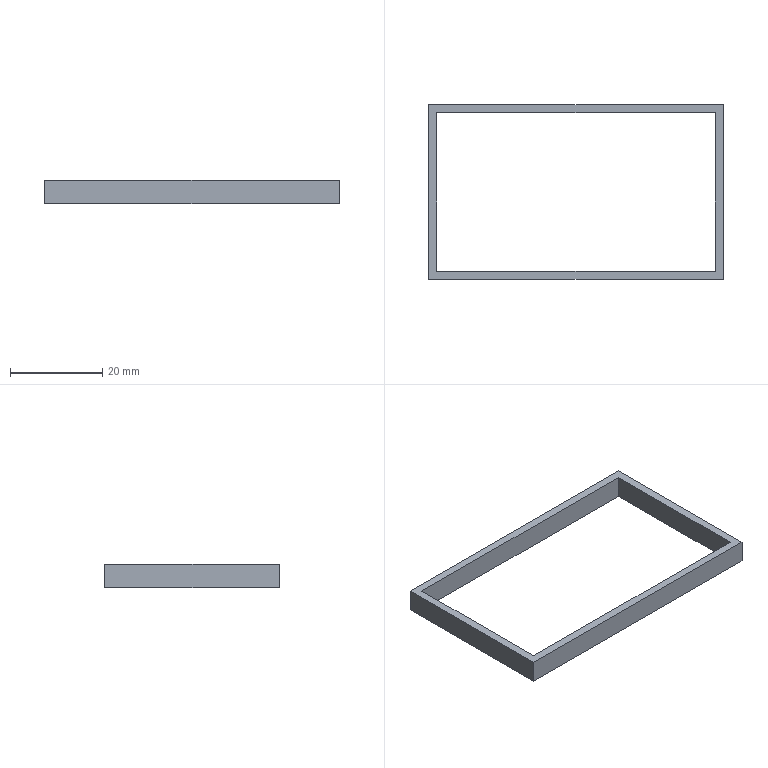Part | SolidWorks | features Extrusion 1 | 1 solid | 10 faces | box 64 x 38 x 5 mm | volume 1771 mm3 | plane 10
STEP:
#1=CARTESIAN_POINT('',(-32.,19.,2.5));
#2=VERTEX_POINT('',#1);
#3=CARTESIAN_POINT('',(-32.,-19.,2.5));
#4=VERTEX_POINT('',#3);
#5=CARTESIAN_POINT('',(-32.,19.,2.5));
#6=DIRECTION('',(0.,-1.,0.));
#7=VECTOR('',#6,1000.);
#8=LINE('',#5,#7);
#9=EDGE_CURVE('',#2,#4,#8,.T.);
#10=ORIENTED_EDGE('',*,*,#9,.F.);
#11=CARTESIAN_POINT('',(-32.,19.,-2.5));
#12=VERTEX_POINT('',#11);
#13=CARTESIAN_POINT('',(-32.,19.,-2.5));
#14=DIRECTION('',(0.,0.,1.));
#15=VECTOR('',#14,1000.);
#16=LINE('',#13,#15);
#17=EDGE_CURVE('',#12,#2,#16,.T.);
#18=ORIENTED_EDGE('',*,*,#17,.F.);
#19=CARTESIAN_POINT('',(-32.,-19.,-2.5));
#20=VERTEX_POINT('',#19);
#21=CARTESIAN_POINT('',(-32.,19.,-2.5));
#22=DIRECTION('',(0.,-1.,0.));
#23=VECTOR('',#22,1000.);
#24=LINE('',#21,#23);
#25=EDGE_CURVE('',#12,#20,#24,.T.);
#26=ORIENTED_EDGE('',*,*,#25,.T.);
#27=CARTESIAN_POINT('',(-32.,-19.,-2.5));
#28=DIRECTION('',(0.,0.,1.));
#29=VECTOR('',#28,1000.);
#30=LINE('',#27,#29);
#31=EDGE_CURVE('',#20,#4,#30,.T.);
#32=ORIENTED_EDGE('',*,*,#31,.T.);
#33=EDGE_LOOP('',(#10,#18,#26,#32));
#34=FACE_OUTER_BOUND('',#33,.T.);
#35=CARTESIAN_POINT('',(-32.,19.,-2.5));
#36=DIRECTION('',(-1.,0.,0.));
#37=DIRECTION('',(0.,0.,1.));
#38=AXIS2_PLACEMENT_3D('',#35,#36,#37);
#39=PLANE('',#38);
#40=ADVANCED_FACE('',(#34),#39,.T.);
#41=CARTESIAN_POINT('',(32.,19.,2.5));
#42=VERTEX_POINT('',#41);
#43=CARTESIAN_POINT('',(32.,19.,2.5));
#44=DIRECTION('',(-1.,0.,0.));
#45=VECTOR('',#44,1000.);
#46=LINE('',#43,#45);
#47=EDGE_CURVE('',#42,#2,#46,.T.);
#48=ORIENTED_EDGE('',*,*,#47,.F.);
#49=CARTESIAN_POINT('',(32.,19.,-2.5));
#50=VERTEX_POINT('',#49);
#51=CARTESIAN_POINT('',(32.,19.,-2.5));
#52=DIRECTION('',(0.,0.,1.));
#53=VECTOR('',#52,1000.);
#54=LINE('',#51,#53);
#55=EDGE_CURVE('',#50,#42,#54,.T.);
#56=ORIENTED_EDGE('',*,*,#55,.F.);
#57=CARTESIAN_POINT('',(32.,19.,-2.5));
#58=DIRECTION('',(-1.,0.,0.));
#59=VECTOR('',#58,1000.);
#60=LINE('',#57,#59);
#61=EDGE_CURVE('',#50,#12,#60,.T.);
#62=ORIENTED_EDGE('',*,*,#61,.T.);
#63=ORIENTED_EDGE('',*,*,#17,.T.);
#64=EDGE_LOOP('',(#48,#56,#62,#63));
#65=FACE_OUTER_BOUND('',#64,.T.);
#66=CARTESIAN_POINT('',(32.,19.,-2.5));
#67=DIRECTION('',(0.,1.,0.));
#68=DIRECTION('',(0.,0.,1.));
#69=AXIS2_PLACEMENT_3D('',#66,#67,#68);
#70=PLANE('',#69);
#71=ADVANCED_FACE('',(#65),#70,.T.);
#72=CARTESIAN_POINT('',(32.,-19.,2.5));
#73=VERTEX_POINT('',#72);
#74=CARTESIAN_POINT('',(32.,-19.,2.5));
#75=DIRECTION('',(0.,1.,0.));
#76=VECTOR('',#75,1000.);
#77=LINE('',#74,#76);
#78=EDGE_CURVE('',#73,#42,#77,.T.);
#79=ORIENTED_EDGE('',*,*,#78,.F.);
#80=CARTESIAN_POINT('',(32.,-19.,-2.5));
#81=VERTEX_POINT('',#80);
#82=CARTESIAN_POINT('',(32.,-19.,-2.5));
#83=DIRECTION('',(0.,0.,1.));
#84=VECTOR('',#83,1000.);
#85=LINE('',#82,#84);
#86=EDGE_CURVE('',#81,#73,#85,.T.);
#87=ORIENTED_EDGE('',*,*,#86,.F.);
#88=CARTESIAN_POINT('',(32.,-19.,-2.5));
#89=DIRECTION('',(0.,1.,0.));
#90=VECTOR('',#89,1000.);
#91=LINE('',#88,#90);
#92=EDGE_CURVE('',#81,#50,#91,.T.);
#93=ORIENTED_EDGE('',*,*,#92,.T.);
#94=ORIENTED_EDGE('',*,*,#55,.T.);
#95=EDGE_LOOP('',(#79,#87,#93,#94));
#96=FACE_OUTER_BOUND('',#95,.T.);
#97=CARTESIAN_POINT('',(32.,-19.,-2.5));
#98=DIRECTION('',(1.,0.,0.));
#99=DIRECTION('',(0.,0.,-1.));
#100=AXIS2_PLACEMENT_3D('',#97,#98,#99);
#101=PLANE('',#100);
#102=ADVANCED_FACE('',(#96),#101,.T.);
#103=CARTESIAN_POINT('',(-32.,-19.,2.5));
#104=DIRECTION('',(1.,0.,0.));
#105=VECTOR('',#104,1000.);
#106=LINE('',#103,#105);
#107=EDGE_CURVE('',#4,#73,#106,.T.);
#108=ORIENTED_EDGE('',*,*,#107,.F.);
#109=ORIENTED_EDGE('',*,*,#31,.F.);
#110=CARTESIAN_POINT('',(-32.,-19.,-2.5));
#111=DIRECTION('',(1.,0.,0.));
#112=VECTOR('',#111,1000.);
#113=LINE('',#110,#112);
#114=EDGE_CURVE('',#20,#81,#113,.T.);
#115=ORIENTED_EDGE('',*,*,#114,.T.);
#116=ORIENTED_EDGE('',*,*,#86,.T.);
#117=EDGE_LOOP('',(#108,#109,#115,#116));
#118=FACE_OUTER_BOUND('',#117,.T.);
#119=CARTESIAN_POINT('',(-32.,-19.,-2.5));
#120=DIRECTION('',(0.,-1.,0.));
#121=DIRECTION('',(0.,0.,-1.));
#122=AXIS2_PLACEMENT_3D('',#119,#120,#121);
#123=PLANE('',#122);
#124=ADVANCED_FACE('',(#118),#123,.T.);
#125=CARTESIAN_POINT('',(30.2,17.2,-2.5));
#126=VERTEX_POINT('',#125);
#127=CARTESIAN_POINT('',(-30.2,17.2,-2.5));
#128=VERTEX_POINT('',#127);
#129=CARTESIAN_POINT('',(30.2,17.2,-2.5));
#130=DIRECTION('',(-1.,0.,0.));
#131=VECTOR('',#130,1000.);
#132=LINE('',#129,#131);
#133=EDGE_CURVE('',#126,#128,#132,.T.);
#134=ORIENTED_EDGE('',*,*,#133,.T.);
#135=CARTESIAN_POINT('',(-30.2,-17.2,-2.5));
#136=VERTEX_POINT('',#135);
#137=CARTESIAN_POINT('',(-30.2,17.2,-2.5));
#138=DIRECTION('',(0.,-1.,0.));
#139=VECTOR('',#138,1000.);
#140=LINE('',#137,#139);
#141=EDGE_CURVE('',#128,#136,#140,.T.);
#142=ORIENTED_EDGE('',*,*,#141,.T.);
#143=CARTESIAN_POINT('',(30.2,-17.2,-2.5));
#144=VERTEX_POINT('',#143);
#145=CARTESIAN_POINT('',(-30.2,-17.2,-2.5));
#146=DIRECTION('',(1.,0.,0.));
#147=VECTOR('',#146,1000.);
#148=LINE('',#145,#147);
#149=EDGE_CURVE('',#136,#144,#148,.T.);
#150=ORIENTED_EDGE('',*,*,#149,.T.);
#151=CARTESIAN_POINT('',(30.2,-17.2,-2.5));
#152=DIRECTION('',(0.,1.,0.));
#153=VECTOR('',#152,1000.);
#154=LINE('',#151,#153);
#155=EDGE_CURVE('',#144,#126,#154,.T.);
#156=ORIENTED_EDGE('',*,*,#155,.T.);
#157=EDGE_LOOP('',(#134,#142,#150,#156));
#158=FACE_BOUND('',#157,.T.);
#159=ORIENTED_EDGE('',*,*,#25,.F.);
#160=ORIENTED_EDGE('',*,*,#61,.F.);
#161=ORIENTED_EDGE('',*,*,#92,.F.);
#162=ORIENTED_EDGE('',*,*,#114,.F.);
#163=EDGE_LOOP('',(#159,#160,#161,#162));
#164=FACE_OUTER_BOUND('',#163,.T.);
#165=CARTESIAN_POINT('',(0.,0.,-2.5));
#166=DIRECTION('',(0.,0.,1.));
#167=DIRECTION('',(1.,0.,0.));
#168=AXIS2_PLACEMENT_3D('',#165,#166,#167);
#169=PLANE('',#168);
#170=ADVANCED_FACE('',(#158,#164),#169,.F.);
#171=CARTESIAN_POINT('',(-30.2,17.2,2.5));
#172=VERTEX_POINT('',#171);
#173=CARTESIAN_POINT('',(-30.2,-17.2,2.5));
#174=VERTEX_POINT('',#173);
#175=CARTESIAN_POINT('',(-30.2,17.2,2.5));
#176=DIRECTION('',(0.,-1.,0.));
#177=VECTOR('',#176,1000.);
#178=LINE('',#175,#177);
#179=EDGE_CURVE('',#172,#174,#178,.T.);
#180=ORIENTED_EDGE('',*,*,#179,.F.);
#181=CARTESIAN_POINT('',(30.2,17.2,2.5));
#182=VERTEX_POINT('',#181);
#183=CARTESIAN_POINT('',(30.2,17.2,2.5));
#184=DIRECTION('',(-1.,0.,0.));
#185=VECTOR('',#184,1000.);
#186=LINE('',#183,#185);
#187=EDGE_CURVE('',#182,#172,#186,.T.);
#188=ORIENTED_EDGE('',*,*,#187,.F.);
#189=CARTESIAN_POINT('',(30.2,-17.2,2.5));
#190=VERTEX_POINT('',#189);
#191=CARTESIAN_POINT('',(30.2,-17.2,2.5));
#192=DIRECTION('',(0.,1.,0.));
#193=VECTOR('',#192,1000.);
#194=LINE('',#191,#193);
#195=EDGE_CURVE('',#190,#182,#194,.T.);
#196=ORIENTED_EDGE('',*,*,#195,.F.);
#197=CARTESIAN_POINT('',(-30.2,-17.2,2.5));
#198=DIRECTION('',(1.,0.,0.));
#199=VECTOR('',#198,1000.);
#200=LINE('',#197,#199);
#201=EDGE_CURVE('',#174,#190,#200,.T.);
#202=ORIENTED_EDGE('',*,*,#201,.F.);
#203=EDGE_LOOP('',(#180,#188,#196,#202));
#204=FACE_BOUND('',#203,.T.);
#205=ORIENTED_EDGE('',*,*,#9,.T.);
#206=ORIENTED_EDGE('',*,*,#107,.T.);
#207=ORIENTED_EDGE('',*,*,#78,.T.);
#208=ORIENTED_EDGE('',*,*,#47,.T.);
#209=EDGE_LOOP('',(#205,#206,#207,#208));
#210=FACE_OUTER_BOUND('',#209,.T.);
#211=CARTESIAN_POINT('',(0.,0.,2.5));
#212=DIRECTION('',(0.,0.,1.));
#213=DIRECTION('',(1.,0.,0.));
#214=AXIS2_PLACEMENT_3D('',#211,#212,#213);
#215=PLANE('',#214);
#216=ADVANCED_FACE('',(#204,#210),#215,.T.);
#217=ORIENTED_EDGE('',*,*,#179,.T.);
#218=CARTESIAN_POINT('',(-30.2,-17.2,-2.5));
#219=DIRECTION('',(0.,0.,1.));
#220=VECTOR('',#219,1000.);
#221=LINE('',#218,#220);
#222=EDGE_CURVE('',#136,#174,#221,.T.);
#223=ORIENTED_EDGE('',*,*,#222,.F.);
#224=ORIENTED_EDGE('',*,*,#141,.F.);
#225=CARTESIAN_POINT('',(-30.2,17.2,-2.5));
#226=DIRECTION('',(0.,0.,1.));
#227=VECTOR('',#226,1000.);
#228=LINE('',#225,#227);
#229=EDGE_CURVE('',#128,#172,#228,.T.);
#230=ORIENTED_EDGE('',*,*,#229,.T.);
#231=EDGE_LOOP('',(#217,#223,#224,#230));
#232=FACE_OUTER_BOUND('',#231,.T.);
#233=CARTESIAN_POINT('',(-30.2,17.2,-2.5));
#234=DIRECTION('',(-1.,0.,0.));
#235=DIRECTION('',(0.,0.,1.));
#236=AXIS2_PLACEMENT_3D('',#233,#234,#235);
#237=PLANE('',#236);
#238=ADVANCED_FACE('',(#232),#237,.F.);
#239=ORIENTED_EDGE('',*,*,#187,.T.);
#240=ORIENTED_EDGE('',*,*,#229,.F.);
#241=ORIENTED_EDGE('',*,*,#133,.F.);
#242=CARTESIAN_POINT('',(30.2,17.2,-2.5));
#243=DIRECTION('',(0.,0.,1.));
#244=VECTOR('',#243,1000.);
#245=LINE('',#242,#244);
#246=EDGE_CURVE('',#126,#182,#245,.T.);
#247=ORIENTED_EDGE('',*,*,#246,.T.);
#248=EDGE_LOOP('',(#239,#240,#241,#247));
#249=FACE_OUTER_BOUND('',#248,.T.);
#250=CARTESIAN_POINT('',(30.2,17.2,-2.5));
#251=DIRECTION('',(0.,1.,0.));
#252=DIRECTION('',(0.,0.,1.));
#253=AXIS2_PLACEMENT_3D('',#250,#251,#252);
#254=PLANE('',#253);
#255=ADVANCED_FACE('',(#249),#254,.F.);
#256=ORIENTED_EDGE('',*,*,#195,.T.);
#257=ORIENTED_EDGE('',*,*,#246,.F.);
#258=ORIENTED_EDGE('',*,*,#155,.F.);
#259=CARTESIAN_POINT('',(30.2,-17.2,-2.5));
#260=DIRECTION('',(0.,0.,1.));
#261=VECTOR('',#260,1000.);
#262=LINE('',#259,#261);
#263=EDGE_CURVE('',#144,#190,#262,.T.);
#264=ORIENTED_EDGE('',*,*,#263,.T.);
#265=EDGE_LOOP('',(#256,#257,#258,#264));
#266=FACE_OUTER_BOUND('',#265,.T.);
#267=CARTESIAN_POINT('',(30.2,-17.2,-2.5));
#268=DIRECTION('',(1.,0.,0.));
#269=DIRECTION('',(0.,0.,-1.));
#270=AXIS2_PLACEMENT_3D('',#267,#268,#269);
#271=PLANE('',#270);
#272=ADVANCED_FACE('',(#266),#271,.F.);
#273=ORIENTED_EDGE('',*,*,#201,.T.);
#274=ORIENTED_EDGE('',*,*,#263,.F.);
#275=ORIENTED_EDGE('',*,*,#149,.F.);
#276=ORIENTED_EDGE('',*,*,#222,.T.);
#277=EDGE_LOOP('',(#273,#274,#275,#276));
#278=FACE_OUTER_BOUND('',#277,.T.);
#279=CARTESIAN_POINT('',(-30.2,-17.2,-2.5));
#280=DIRECTION('',(0.,-1.,0.));
#281=DIRECTION('',(0.,0.,-1.));
#282=AXIS2_PLACEMENT_3D('',#279,#280,#281);
#283=PLANE('',#282);
#284=ADVANCED_FACE('',(#278),#283,.F.);
#285=CLOSED_SHELL('',(#40,#71,#102,#124,#170,#216,#238,#255,#272,#284));
#286=MANIFOLD_SOLID_BREP('',#285);
#287=CARTESIAN_POINT('',(0.,0.,0.));
#288=DIRECTION('',(0.,0.,1.));
#289=DIRECTION('',(1.,0.,0.));
#290=AXIS2_PLACEMENT_3D('',#287,#288,#289);
#291=(LENGTH_UNIT()NAMED_UNIT(*)SI_UNIT(.MILLI.,.METRE.));
#292=UNCERTAINTY_MEASURE_WITH_UNIT(LENGTH_MEASURE(0.00001),#291,'','');
#293=(NAMED_UNIT(*)PLANE_ANGLE_UNIT()SI_UNIT($,.RADIAN.));
#294=(NAMED_UNIT(*)SI_UNIT($,.STERADIAN.)SOLID_ANGLE_UNIT());
#295=(GEOMETRIC_REPRESENTATION_CONTEXT(3)GLOBAL_UNCERTAINTY_ASSIGNED_CONTEXT((#292))GLOBAL_UNIT_ASSIGNED_CONTEXT((#291,#293,#294))REPRESENTATION_CONTEXT('',''));
#296=ADVANCED_BREP_SHAPE_REPRESENTATION('',(#286,#290),#295);